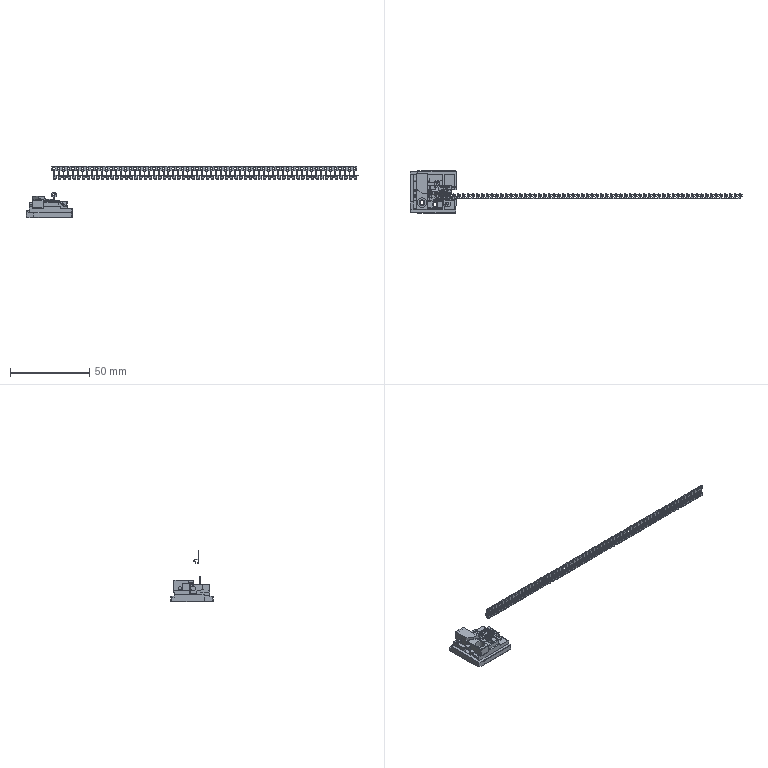Part | NX | 12 solids | 8364 faces | volume 5164 mm3 | plane 3737 | cylinder 2907 | torus 1362 | sphere 308 | cone 28 | spline 22 | commonest cylinder face diameters 0.2 x628 0.8 x335 0.4 x281 0.6 x266 0.12 x260 0.44 x260